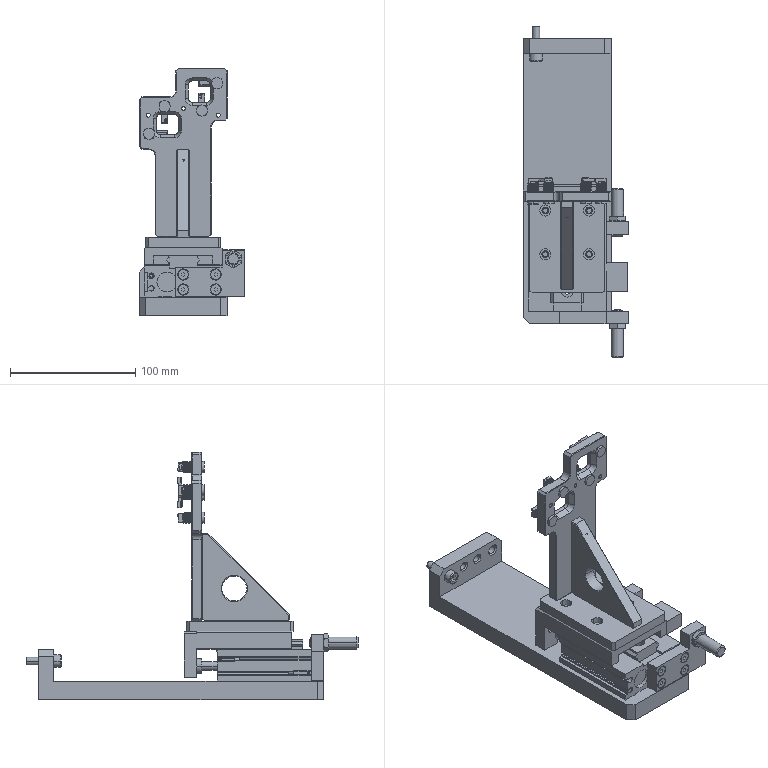Part | SolidWorks | features InContextFeatHolder 2, Attribute 1 | 32 solids | 1372 faces | box 84 x 265.5 x 198 mm | volume 582141 mm3 | plane 758 | cylinder 362 | cone 196 | spline 38 | sphere 12 | torus 6 | commonest cylinder face diameters 9 x40 4 x29 1.5 x28 4.134 x28 5 x27 6 x18